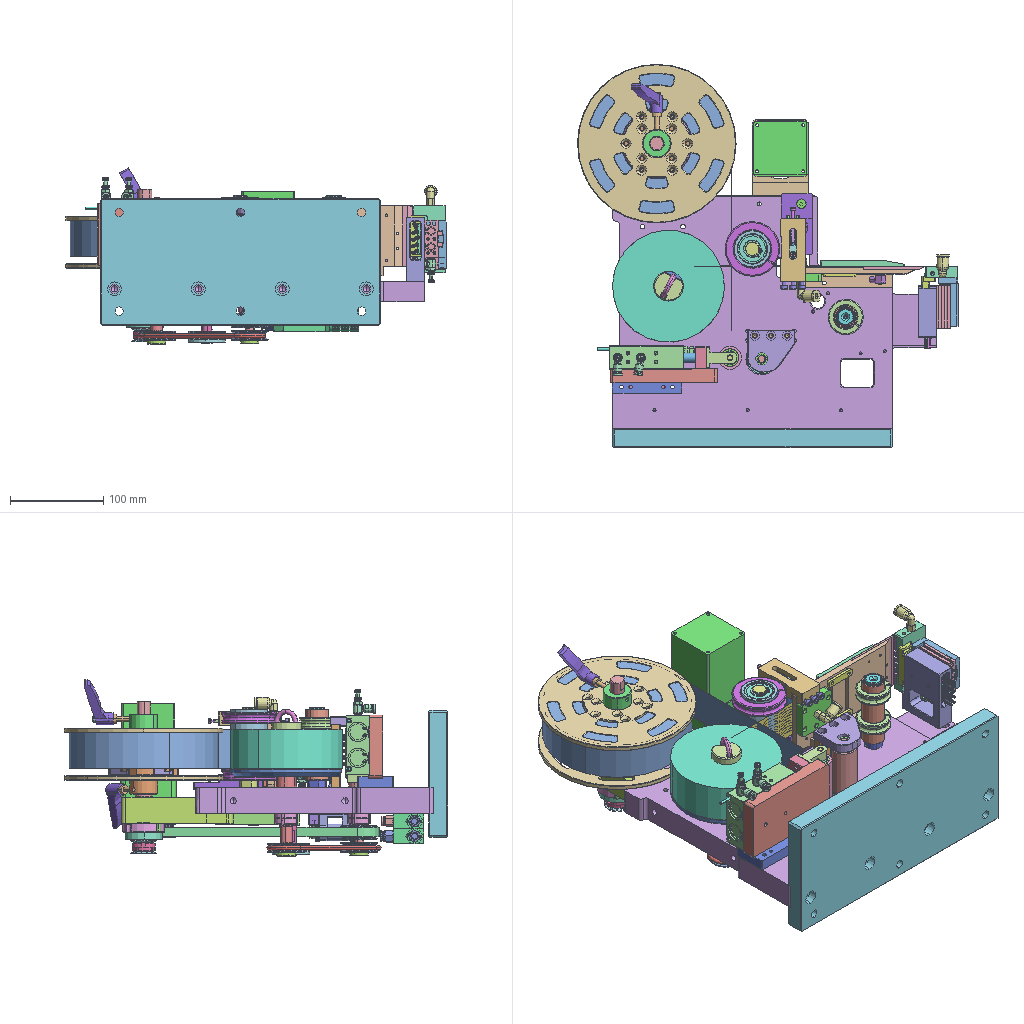Assembly | STEP file | 101 different items | 156 placed | box 409 x 411 x 189 mm
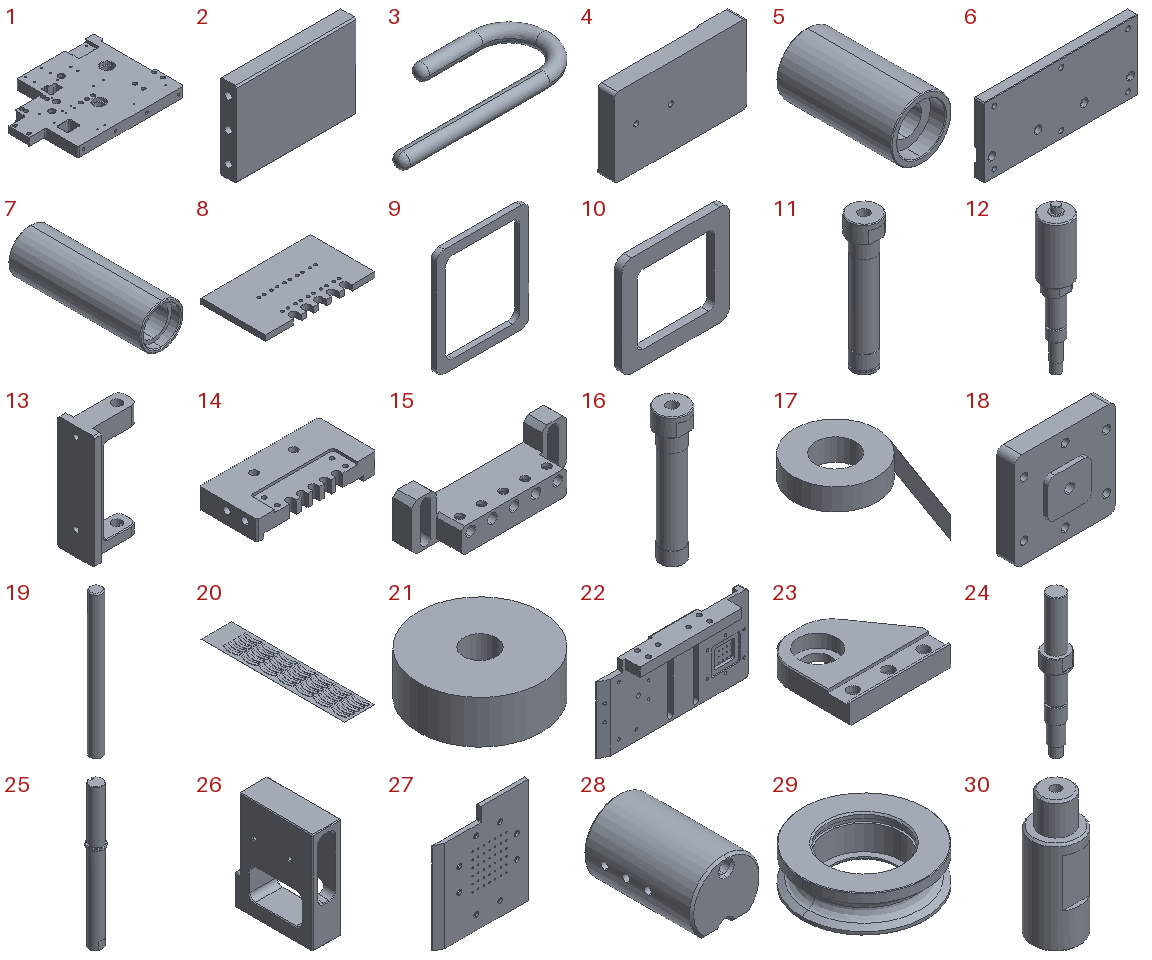Parts list (item | name | quantity | parent item | size | volume):
1 | 10000020440swp000-1 | x1 | in Label stripping machine | 348 x 255 x 28 mm | 1845671 mm3
2 | 10000020443swp000-1 | x1 | in 10000020438swa000-1 | 70.5 x 10 x 50 mm | 33628 mm3
3 | 10000020444swp000-1 | x1 | in 10000020498swa000-1 | 62.75 x 27.5 x 5 mm | 2027 mm3
4 | 10000020445swp000-1 | x1 | in 10000020495swa000-1 | 115 x 15 x 68 mm | 111374 mm3
5 | 10000020449swp000-1 | x1 | in 10000020462swa000-1 | 40 x 76 x 40 mm | 61770 mm3
6 | 10000020450swp000-1 | x1 | in Label stripping machine | 300 x 20 x 136 mm | 751021 mm3
7 | 10000020451swp000-1 | x1 | in 10000020490swa000-1 | 25 x 76 x 25 mm | 18826 mm3
8 | 10000020453swp000-1 | x1 | in 10000020477swa000(Default -_flexible1) | 60 x 35 x 3 mm | 5964 mm3
9 | 10000020458swp000-1 | x1 | in 10000020482swa000(Default -_flexible1) | 36 x 2 x 42 mm | 994 mm3
10 | 10000020460swp000-1 | x1 | in 10000020482swa000(Default -_flexible1) | 28 x 2 x 26 mm | 729.133 mm3
11 | 10000020461swp000-1 | x1 | in 10000020462swa000-1 | 20 x 20 x 89 mm | 15653 mm3
12 | 10000020465swp000-1 | x1 | in 10000020438swa000-1 | 28.65 x 28.65 x 140.9 mm | 48218 mm3
13 | 10000020470swp000-1 | x1 | in 10000020495swa000-1 | 32.5 x 23 x 71 mm | 16585 mm3
14 | 10000020471swp000-1 | x1 | in 10000020477swa000(Default -_flexible1) | 72 x 35 x 12 mm | 19636 mm3
15 | 10000020473swp000-1 | x1 | in 10000020477swa000(Default -_flexible1) | 50 x 14 x 15 mm | 4019 mm3
16 | 10000020474swp000-1 | x1 | in 10000020490swa000-1 | 20 x 20 x 86 mm | 15036 mm3
17 | 10000020479swp000-1 | x1 | in 10000020457swa000-1 | 160 x 295.688 x 42 mm | 654576 mm3
18 | 10000020483swp000-1 | x1 | in 10000020482swa000(Default -_flexible1) | 44 x 10 x 42 mm | 14387 mm3
19 | 10000020485swp000-1 | x1 | in 10000020495swa000-1 | 6 x 6 x 71 mm | 1989 mm3
20 | 10000020486swp000-1 | x1 | in Label stripping machine | 42 x 200 x 0.9 mm | 2989 mm3
21 | 10000020487swp000-1 | x1 | in 10000020498swa000-1 | 120 x 120 x 42 mm | 441230 mm3
22 | 10000020488swp000-1 | x1 | in 10000020482swa000(Default -_flexible1) | 144 x 22 x 75 mm | 68322 mm3
23 | 10000020492swp000-1 | x1 | in 10000020438swa000-1 | 50 x 45 x 10 mm | 14150 mm3
24 | 10000020499swp000-1 | x1 | in 10000020498swa000-1 | 22 x 22 x 126.85 mm | 22513 mm3
25 | 10000020500swp000-1 | x1 | in 10000020457swa000-1 | 18 x 18 x 163 mm | 28114 mm3
26 | 10000020502swp000-1 | x1 | in 10000020477swa000(Default -_flexible1) | 20 x 55 x 71.5 mm | 35997 mm3
27 | 10000020503swp000-1 | x1 | in 10000020482swa000(Default -_flexible1) | 66 x 3 x 75 mm | 12831 mm3
28 | 10000020504swp000-1 | x1 | in 10000020498swa000-1 | 32 x 50 x 28 mm | 27586 mm3
29 | 10000020541swp000-1 | x1 | in 10000020556swa000-1 | 40 x 40 x 12 mm | 7266 mm3
30 | 10000020542swp000-1 | x1 | in 10000020556swa000-1 | 12 x 12 x 31.5 mm | 2667 mm3
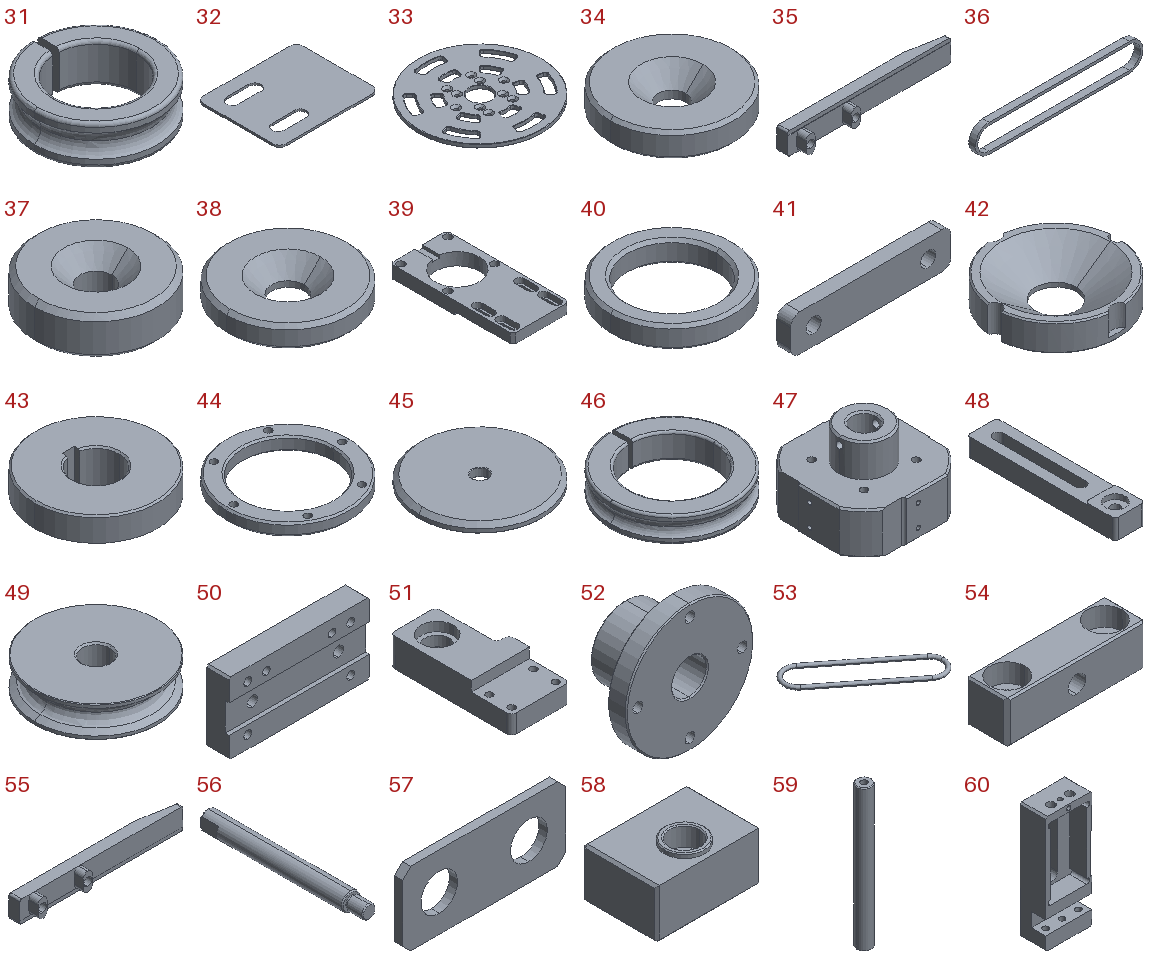31 | 10000020543swp000-1 | x2 | in 10000020490swa000-1 | 37.8 x 37.774 x 12 mm | 6334 mm3
32 | 10000020545swp000-1 | x4 | in 10000020457swa000-1 | 29 x 24 x 0.6 mm | 376.694 mm3
33 | 10000020546swp000-1 | x2 | in 10000020457swa000-1 | 170 x 170 x 5 mm | 86997 mm3
34 | 10000020547swp000-1 | x2 | in 10000020438swa000-1, 10000020498swa000-1 | 20 x 20 x 4 mm | 1102 mm3
35 | 10000020548swp000-1 | x1 | in 10000020482swa000(Default -_flexible1) | 90 x 11 x 12 mm | 5809 mm3
36 | 10000020550swp000-1 | x1 | in Label stripping machine | 260.44 x 10 x 43.01 mm | 22297 mm3
37 | 10000020551swp000-1 | x1 | in 10000020556swa000-1 | 13 x 13 x 4 mm | 465.157 mm3
38 | 10000020557swp000-1 | x1 | in 10000020490swa000-1 | 17 x 17 x 3 mm | 573.373 mm3
39 | 10000020558swp000-1 | x1 | in 10000020472swa000-1 | 60 x 130 x 13 mm | 60488 mm3
40 | 10000020559swp000-1 | x2 | in 10000020495swa000-1 | 8.5 x 8.5 x 1.5 mm | 39.446 mm3
41 | 10000020560swp000-1 | x2 | in 10000020482swa000(Default -_flexible1) | 35 x 3 x 8 mm | 778.381 mm3
42 | 10000020561swp000-1 | x1 | in 10000020457swa000-1 | 44.722 x 45 x 10 mm | 10014 mm3
43 | 10000020570swp000-1 | x1 | in 10000020457swa000-1 | 40 x 40 x 14 mm | 11944 mm3
44 | 10000020571swp000-1 | x1 | in 10000020457swa000-1 | 75 x 75 x 8 mm | 14917 mm3
45 | 10000020576swp000-1 | x1 | in 10000020498swa000-1 | 120 x 120 x 8 mm | 86018 mm3
46 | 10000020578swp000-1 | x2 | in 10000020462swa000-1 | 58.8 x 58.783 x 12 mm | 15552 mm3
47 | 10000020580swp000-1 | x1 | in 10000020457swa000-1 | 66 x 66 x 45.5 mm | 104414 mm3
48 | 10000020588swp000-1 | x1 | in 10000020556swa000-1 | 18 x 90 x 12 mm | 13483 mm3
49 | 10000020591swp000-1 | x2 | in 10000020438swa000-1, 10000020498swa000-1 | 40 x 40 x 10 mm | 9487 mm3
50 | 10000020593swp000-1 | x1 | in 10000020495swa000-1 | 75 x 12 x 38 mm | 29849 mm3
51 | 10000020597swp000-1 | x1 | in 10000020457swa000-1 | 57.5 x 120 x 28 mm | 124322 mm3
52 | 10000020598swp000-1 | x1 | in 10000020457swa000-1 | 55 x 28 x 55 mm | 27477 mm3
53 | 10000020599swp000-1 | x1 | in Label stripping machine | 141 x 119 x 5 mm | 7201 mm3
54 | 10000020605swp000-1 | x2 | in 10000020472swa000-1, 10000020556swa000-1 | 40 x 12 x 12 mm | 4314 mm3
55 | 10000020606swp000-1 | x1 | in 10000020482swa000(Default -_flexible1) | 90 x 11 x 12 mm | 5783 mm3
56 | 10000054026swp000-1 | x4 | in 10000054270swa000-1 | 4 x 36 x 4 mm | 421.312 mm3
57 | 10000054028swp000-1 | x2 | in 10000054270swa000-1 | 20 x 1 x 9 mm | 146.191 mm3
58 | 10000054265swp000-1 | x2 | in 10000054270swa000-1 | 21 x 15 x 10.9 mm | 2839 mm3
59 | 10000054268swp000-1 | x1 | in 10000054270swa000-1 | 6 x 6 x 58 mm | 1518 mm3
60 | 10000054277swp000-1 | x1 | in 10000054270swa000-1 | 27 x 15 x 68 mm | 14711 mm3
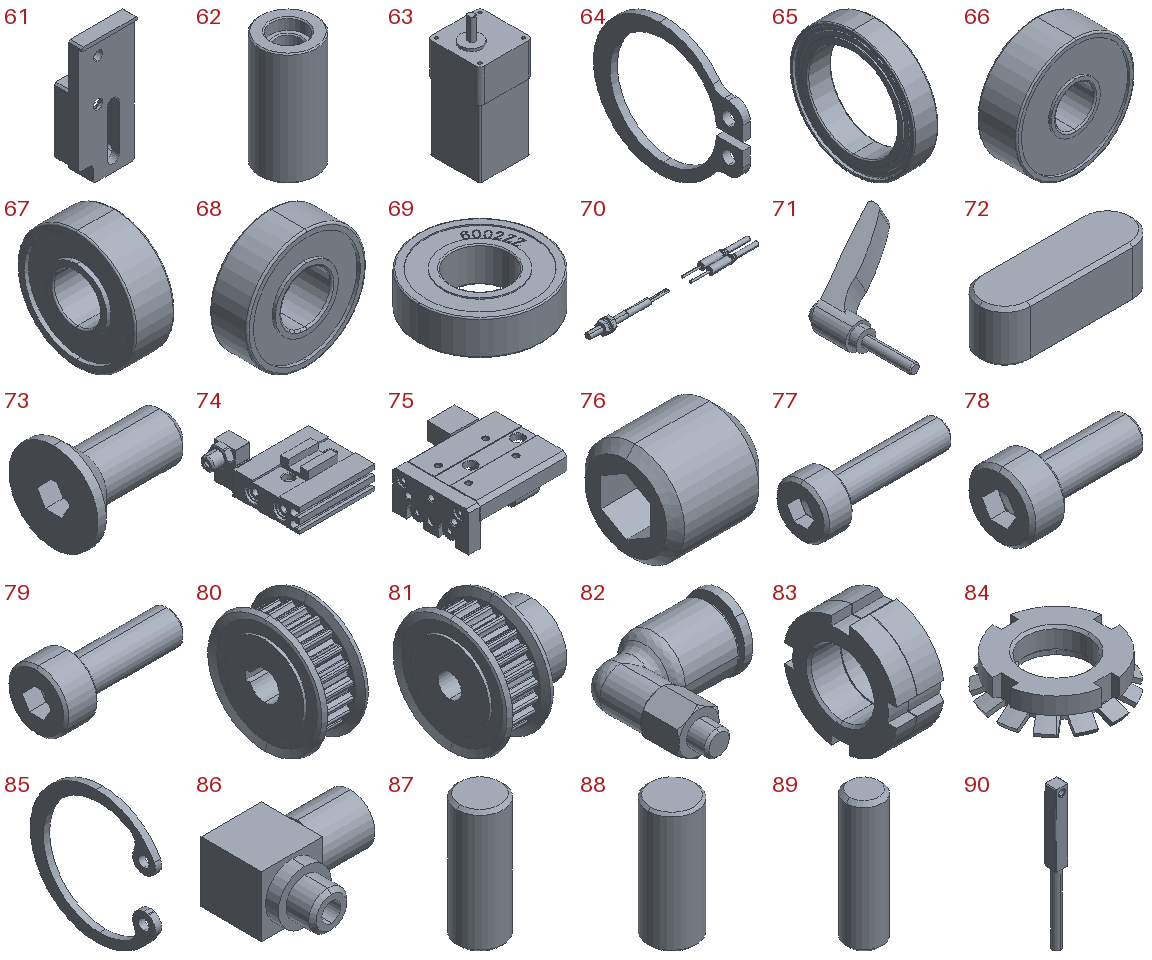61 | 10000054304swp000-1 | x1 | in 10000054270swa000-1 | 33 x 16.5 x 75 mm | 16269 mm3
62 | 10000054363swp000-1 | x1 | in 10000054270swa000-1 | 25 x 25 x 50 mm | 18935 mm3
63 | 57BYG gear reduction stepper motor Mingren MR57BYG76-P10-1 | x1 | in 10000020472swa000-1 | 60 x 60 x 143 mm | 384480 mm3
64 | C-type retaining ring MISUMI STWN15-1 | x1 | in 10000020462swa000-1 | 1 x 20 x 17.6 mm | 97.521 mm3
65 | Deep groove ball bearing NSK SB6702ZZ-1 | x2 | in 10000020490swa000-1 | 4 x 21 x 21 mm | 419.102 mm3
66 | Domestic miniature ball bearing NSK 628ZZ-1 | x1 | in 10000020556swa000-1 | 24 x 8 x 24 mm | 2912 mm3
67 | Domestic miniature ball bearing NSK 696ZZ1-1 | x2 | in 10000054270swa000-1 | 5 x 15 x 15 mm | 647.818 mm3
68 | Domestic miniature ball bearing NSK 698ZZ-1 | x1 | in 10000020438swa000-1 | 19 x 6 x 19 mm | 1248 mm3
69 | Domestic single-row deep groove ball bearing NSK 6002ZZ-1 | x8 | in 10000020438swa000-1, 10000020457swa000-1, 10000020462swa000-1, 10000020498swa000-1 | 32 x 32 x 9 mm | 5439 mm3
70 | Fiber optic sensor OMRON E32-ZC31 straight coaxial sensing distance 7mm-1 | x5 | in 10000020477swa000(Default -_flexible1) | - | -
71 | Fixed handle MISUMI CLDM5-25-B-1 | x2 | in 10000020457swa000-1 | - | -
72 | Flat key Shanglong KEA-B4-L12-1 | x2 | in 10000020438swa000-1, 10000020457swa000-1 | 12 x 4 x 4 mm | 176.513 mm3
73 | Flat-head hex socket screw Dongming full thread M5-12 A2-70-1 | x2 | in 10000054270swa000-1 | 12 x 9.43 x 9.43 mm | 310.666 mm3
74 | HLQ8-10-S-AS-1-1 | x1 | in Precision slide cylinder AirTAC HLQ8-10-S-AS-1 | 54.5 x 53.15 x 23 mm | 23143 mm3
75 | HLQ8-10-S-AS-2-1 | x1 | in Precision slide cylinder AirTAC HLQ8-10-S-AS-1 | 52 x 51.5 x 21 mm | 19231 mm3
76 | Headless hex socket screw Dongming full thread M3-3 A2-70-1 | x2 | in 10000054270swa000-1 | 3 x 3 x 3 mm | 17.241 mm3
77 | Hex socket screw Dongming full thread M3-12 A2-70-1 | x2 | in 10000054270swa000-1 | 15 x 5.68 x 5.68 mm | 150.677 mm3
78 | Hex socket screw Dongming full thread M3-8 A2-70-1 | x2 | in 10000054270swa000-1 | 11 x 5.68 x 5.68 mm | 122.403 mm3
79 | Hex socket screw Dongming full thread M4-12 A2-70-1 | x3 | in 10000054270swa000-1 | 16 x 7.22 x 7.22 mm | 294.412 mm3
80 | High-torque timing pulley MISUMI HTPA22S5M100-A-N10-1 | x1 | in 10000020438swa000-1 | - | -
81 | High-torque timing pulley MISUMI HTPA22S5M100-B-P8-1 | x1 | in 10000020472swa000-1 | - | -
82 | L-type threaded two-way connector Yiri EGPL6-M5-1 | x2 | in 10000020477swa000(Default -_flexible1), 10000020482swa000(Default -_flexible1) | - | -
83 | Lock nut MISUMI FUNT15-1 | x2 | in 10000020438swa000-1, 10000020498swa000-1 | 11.5 x 24.678 x 24.678 mm | 3349 mm3
84 | Lock nut MISUMI JLNK15-1 | x2 | in 10000020457swa000-1 | 27.99 x 27.99 x 7.435 mm | 1826 mm3
85 | MISUMI C-type retaining ring RTWN24-1 | x1 | in 10000020556swa000-1 | 1.2 x 23.885 x 25.2 mm | 171.114 mm3
86 | Miniature fitting SMC M-5HL-4-1 | x1 | in 10000020482swa000(Default -_flexible1) | - | -
87 | Needle roller domestic φ3-8-1 | x2 | in 10000020477swa000(Default -_flexible1) | 3 x 3 x 8 mm | 56.188 mm3
88 | Needle roller domestic φ4-10-1 | x4 | in 10000020482swa000(Default -_flexible1), 10000020495swa000-1 | 4 x 4 x 10 mm | 125.178 mm3
89 | Needle roller domestic φ5-18-1 | x2 | in 10000020457swa000-1 | 5 x 5 x 18 mm | 349.764 mm3
90 | Proximity switch AirTAC DS1-G-020-1 | x2 | in 10000020495swa000-1 | 4.4 x 5 x 50.8 mm | 677.466 mm3
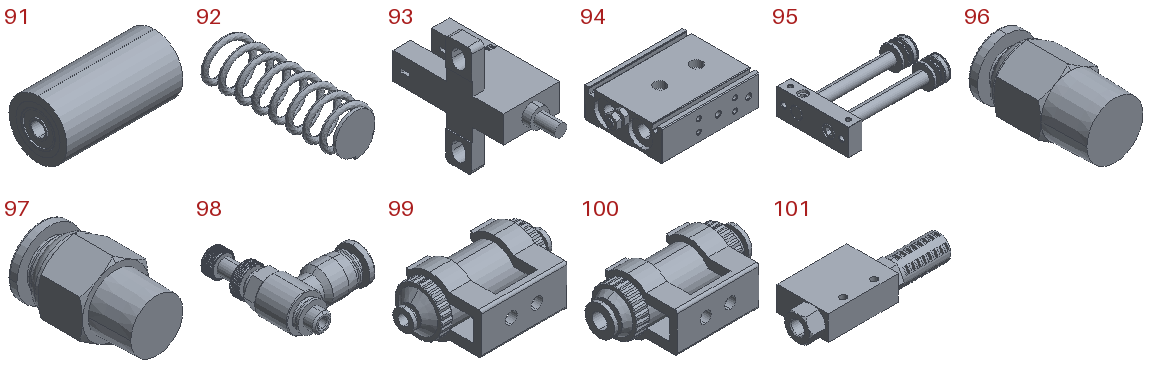91 | Roller MISUMI RORJA25-50-1 | x1 | in 10000020495swa000-1 | - | -
92 | Round wire coil spring Katalo FUR8-25-B-1 | x4 | in 10000054270swa000-1 | 8 x 24.5 x 8 mm | 156.394 mm3
93 | Sensor OMRON EE-SX672-WR-1 | x1 | in 10000020482swa000(Default -_flexible1) | 13.7 x 33.2 x 26 mm | 2293 mm3
94 | TR20-10-S-1-1 | x1 | in Twin-rod cylinder AirTAC TR20-10-S-1 | - | -
95 | TR20-10-S-2-1 | x1 | in Twin-rod cylinder AirTAC TR20-10-S-1 | - | -
96 | Threaded straight connector Yiri EPC4-01-1 | x1 | in 10000020475swa000(Default -_flexible1) | - | -
97 | Threaded straight connector Yiri EPC6-01-1 | x3 | in 10000020475swa000(Default -_flexible1) | - | -
98 | Tube-fitting one-way flow control valve AirTAC ASL4-M5-1 | x4 | in 10000020477swa000(Default -_flexible1), 10000020495swa000-1 | 23.8 x 30 x 9.8 mm | 1827 mm3
99 | Vacuum filter Qilike VFD-02-04-1 | x1 | in 10000020475swa000(Default -_flexible1) | 53.5 x 29.25 x 22 mm | 14857 mm3
100 | Vacuum filter Qilike VFD-02-06-1 | x1 | in 10000020475swa000(Default -_flexible1) | 55.5 x 29.25 x 22 mm | 15469 mm3
101 | Vacuum generator Qilike EV-10-1 | x2 | in 10000020475swa000(Default -_flexible1) | - | -